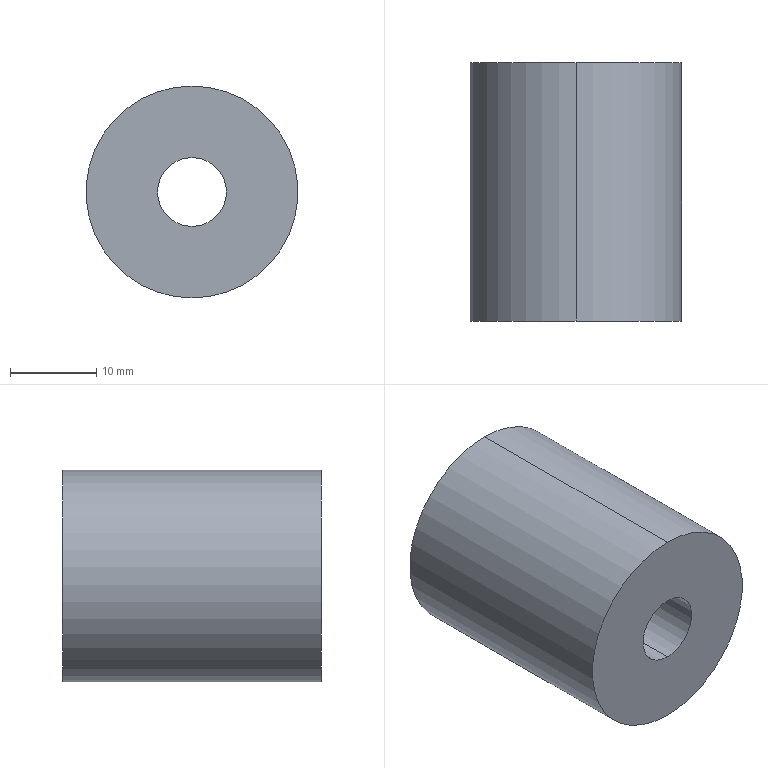Part | SolidWorks | features Revolution 1 | 1 solid | 6 faces | box 24.6 x 30 x 24.6 mm | volume 12751 mm3 | cylinder 4 | plane 2 | commonest cylinder face diameters 8 x2 24.6 x2
STEP:
#1=CARTESIAN_POINT('',(0.,25.747,-12.3));
#2=VERTEX_POINT('',#1);
#3=CARTESIAN_POINT('',(0.,25.747,12.3));
#4=VERTEX_POINT('',#3);
#5=CARTESIAN_POINT('',(0.,25.747,0.));
#6=DIRECTION('',(0.,-1.,0.));
#7=DIRECTION('',(0.,0.,-1.));
#8=AXIS2_PLACEMENT_3D('',#5,#6,#7);
#9=CIRCLE('',#8,12.3);
#10=EDGE_CURVE('',#2,#4,#9,.T.);
#11=ORIENTED_EDGE('',*,*,#10,.T.);
#12=CARTESIAN_POINT('',(0.,-4.253,12.3));
#13=VERTEX_POINT('',#12);
#14=CARTESIAN_POINT('',(0.,0.,12.3));
#15=DIRECTION('',(0.,-1.,0.));
#16=VECTOR('',#15,1000.);
#17=LINE('',#14,#16);
#18=EDGE_CURVE('',#4,#13,#17,.T.);
#19=ORIENTED_EDGE('',*,*,#18,.T.);
#20=CARTESIAN_POINT('',(0.,-4.253,-12.3));
#21=VERTEX_POINT('',#20);
#22=CARTESIAN_POINT('',(0.,-4.253,0.));
#23=DIRECTION('',(0.,-1.,0.));
#24=DIRECTION('',(0.,0.,-1.));
#25=AXIS2_PLACEMENT_3D('',#22,#23,#24);
#26=CIRCLE('',#25,12.3);
#27=EDGE_CURVE('',#21,#13,#26,.T.);
#28=ORIENTED_EDGE('',*,*,#27,.F.);
#29=CARTESIAN_POINT('',(0.,0.,-12.3));
#30=DIRECTION('',(0.,-1.,0.));
#31=VECTOR('',#30,1000.);
#32=LINE('',#29,#31);
#33=EDGE_CURVE('',#2,#21,#32,.T.);
#34=ORIENTED_EDGE('',*,*,#33,.F.);
#35=EDGE_LOOP('',(#11,#19,#28,#34));
#36=FACE_OUTER_BOUND('',#35,.T.);
#37=CARTESIAN_POINT('',(0.,0.,0.));
#38=DIRECTION('',(0.,-1.,0.));
#39=DIRECTION('',(0.,0.,-1.));
#40=AXIS2_PLACEMENT_3D('',#37,#38,#39);
#41=CYLINDRICAL_SURFACE('',#40,12.3);
#42=ADVANCED_FACE('',(#36),#41,.T.);
#43=CARTESIAN_POINT('',(0.,25.747,4.));
#44=VERTEX_POINT('',#43);
#45=CARTESIAN_POINT('',(0.,25.747,-4.));
#46=VERTEX_POINT('',#45);
#47=CARTESIAN_POINT('',(0.,25.747,0.));
#48=DIRECTION('',(0.,-1.,0.));
#49=DIRECTION('',(0.,0.,-1.));
#50=AXIS2_PLACEMENT_3D('',#47,#48,#49);
#51=CIRCLE('',#50,4.);
#52=EDGE_CURVE('',#44,#46,#51,.T.);
#53=ORIENTED_EDGE('',*,*,#52,.F.);
#54=CARTESIAN_POINT('',(0.,-4.253,4.));
#55=VERTEX_POINT('',#54);
#56=CARTESIAN_POINT('',(0.,0.,4.));
#57=DIRECTION('',(0.,-1.,0.));
#58=VECTOR('',#57,1000.);
#59=LINE('',#56,#58);
#60=EDGE_CURVE('',#44,#55,#59,.T.);
#61=ORIENTED_EDGE('',*,*,#60,.T.);
#62=CARTESIAN_POINT('',(0.,-4.253,-4.));
#63=VERTEX_POINT('',#62);
#64=CARTESIAN_POINT('',(0.,-4.253,0.));
#65=DIRECTION('',(0.,-1.,0.));
#66=DIRECTION('',(0.,0.,-1.));
#67=AXIS2_PLACEMENT_3D('',#64,#65,#66);
#68=CIRCLE('',#67,4.);
#69=EDGE_CURVE('',#55,#63,#68,.T.);
#70=ORIENTED_EDGE('',*,*,#69,.T.);
#71=CARTESIAN_POINT('',(0.,0.,-4.));
#72=DIRECTION('',(0.,-1.,0.));
#73=VECTOR('',#72,1000.);
#74=LINE('',#71,#73);
#75=EDGE_CURVE('',#46,#63,#74,.T.);
#76=ORIENTED_EDGE('',*,*,#75,.F.);
#77=EDGE_LOOP('',(#53,#61,#70,#76));
#78=FACE_OUTER_BOUND('',#77,.T.);
#79=CARTESIAN_POINT('',(0.,0.,0.));
#80=DIRECTION('',(0.,-1.,0.));
#81=DIRECTION('',(0.,0.,-1.));
#82=AXIS2_PLACEMENT_3D('',#79,#80,#81);
#83=CYLINDRICAL_SURFACE('',#82,4.);
#84=ADVANCED_FACE('',(#78),#83,.F.);
#85=ORIENTED_EDGE('',*,*,#60,.F.);
#86=CARTESIAN_POINT('',(0.,25.747,0.));
#87=DIRECTION('',(0.,-1.,0.));
#88=DIRECTION('',(0.,0.,-1.));
#89=AXIS2_PLACEMENT_3D('',#86,#87,#88);
#90=CIRCLE('',#89,4.);
#91=EDGE_CURVE('',#46,#44,#90,.T.);
#92=ORIENTED_EDGE('',*,*,#91,.F.);
#93=ORIENTED_EDGE('',*,*,#75,.T.);
#94=CARTESIAN_POINT('',(0.,-4.253,0.));
#95=DIRECTION('',(0.,-1.,0.));
#96=DIRECTION('',(0.,0.,-1.));
#97=AXIS2_PLACEMENT_3D('',#94,#95,#96);
#98=CIRCLE('',#97,4.);
#99=EDGE_CURVE('',#63,#55,#98,.T.);
#100=ORIENTED_EDGE('',*,*,#99,.T.);
#101=EDGE_LOOP('',(#85,#92,#93,#100));
#102=FACE_OUTER_BOUND('',#101,.T.);
#103=CARTESIAN_POINT('',(0.,0.,0.));
#104=DIRECTION('',(0.,-1.,0.));
#105=DIRECTION('',(0.,0.,-1.));
#106=AXIS2_PLACEMENT_3D('',#103,#104,#105);
#107=CYLINDRICAL_SURFACE('',#106,4.);
#108=ADVANCED_FACE('',(#102),#107,.F.);
#109=ORIENTED_EDGE('',*,*,#91,.T.);
#110=ORIENTED_EDGE('',*,*,#52,.T.);
#111=EDGE_LOOP('',(#109,#110));
#112=FACE_BOUND('',#111,.T.);
#113=ORIENTED_EDGE('',*,*,#10,.F.);
#114=CARTESIAN_POINT('',(0.,25.747,0.));
#115=DIRECTION('',(0.,-1.,0.));
#116=DIRECTION('',(0.,0.,-1.));
#117=AXIS2_PLACEMENT_3D('',#114,#115,#116);
#118=CIRCLE('',#117,12.3);
#119=EDGE_CURVE('',#4,#2,#118,.T.);
#120=ORIENTED_EDGE('',*,*,#119,.F.);
#121=EDGE_LOOP('',(#113,#120));
#122=FACE_OUTER_BOUND('',#121,.T.);
#123=CARTESIAN_POINT('',(4.,25.747,0.));
#124=DIRECTION('',(0.,1.,0.));
#125=DIRECTION('',(0.,0.,1.));
#126=AXIS2_PLACEMENT_3D('',#123,#124,#125);
#127=PLANE('',#126);
#128=ADVANCED_FACE('',(#112,#122),#127,.T.);
#129=ORIENTED_EDGE('',*,*,#18,.F.);
#130=ORIENTED_EDGE('',*,*,#119,.T.);
#131=ORIENTED_EDGE('',*,*,#33,.T.);
#132=CARTESIAN_POINT('',(0.,-4.253,0.));
#133=DIRECTION('',(0.,-1.,0.));
#134=DIRECTION('',(0.,0.,-1.));
#135=AXIS2_PLACEMENT_3D('',#132,#133,#134);
#136=CIRCLE('',#135,12.3);
#137=EDGE_CURVE('',#13,#21,#136,.T.);
#138=ORIENTED_EDGE('',*,*,#137,.F.);
#139=EDGE_LOOP('',(#129,#130,#131,#138));
#140=FACE_OUTER_BOUND('',#139,.T.);
#141=CARTESIAN_POINT('',(0.,0.,0.));
#142=DIRECTION('',(0.,-1.,0.));
#143=DIRECTION('',(0.,0.,-1.));
#144=AXIS2_PLACEMENT_3D('',#141,#142,#143);
#145=CYLINDRICAL_SURFACE('',#144,12.3);
#146=ADVANCED_FACE('',(#140),#145,.T.);
#147=ORIENTED_EDGE('',*,*,#27,.T.);
#148=ORIENTED_EDGE('',*,*,#137,.T.);
#149=EDGE_LOOP('',(#147,#148));
#150=FACE_OUTER_BOUND('',#149,.T.);
#151=ORIENTED_EDGE('',*,*,#99,.F.);
#152=ORIENTED_EDGE('',*,*,#69,.F.);
#153=EDGE_LOOP('',(#151,#152));
#154=FACE_BOUND('',#153,.T.);
#155=CARTESIAN_POINT('',(12.3,-4.253,0.));
#156=DIRECTION('',(0.,-1.,0.));
#157=DIRECTION('',(0.,0.,-1.));
#158=AXIS2_PLACEMENT_3D('',#155,#156,#157);
#159=PLANE('',#158);
#160=ADVANCED_FACE('',(#150,#154),#159,.T.);
#161=CLOSED_SHELL('',(#42,#84,#108,#128,#146,#160));
#162=MANIFOLD_SOLID_BREP('',#161);
#163=CARTESIAN_POINT('',(0.,0.,0.));
#164=DIRECTION('',(0.,0.,1.));
#165=DIRECTION('',(1.,0.,0.));
#166=AXIS2_PLACEMENT_3D('',#163,#164,#165);
#167=(LENGTH_UNIT()NAMED_UNIT(*)SI_UNIT(.MILLI.,.METRE.));
#168=UNCERTAINTY_MEASURE_WITH_UNIT(LENGTH_MEASURE(0.00001),#167,'','');
#169=(NAMED_UNIT(*)PLANE_ANGLE_UNIT()SI_UNIT($,.RADIAN.));
#170=(NAMED_UNIT(*)SI_UNIT($,.STERADIAN.)SOLID_ANGLE_UNIT());
#171=(GEOMETRIC_REPRESENTATION_CONTEXT(3)GLOBAL_UNCERTAINTY_ASSIGNED_CONTEXT((#168))GLOBAL_UNIT_ASSIGNED_CONTEXT((#167,#169,#170))REPRESENTATION_CONTEXT('',''));
#172=ADVANCED_BREP_SHAPE_REPRESENTATION('',(#162,#166),#171);